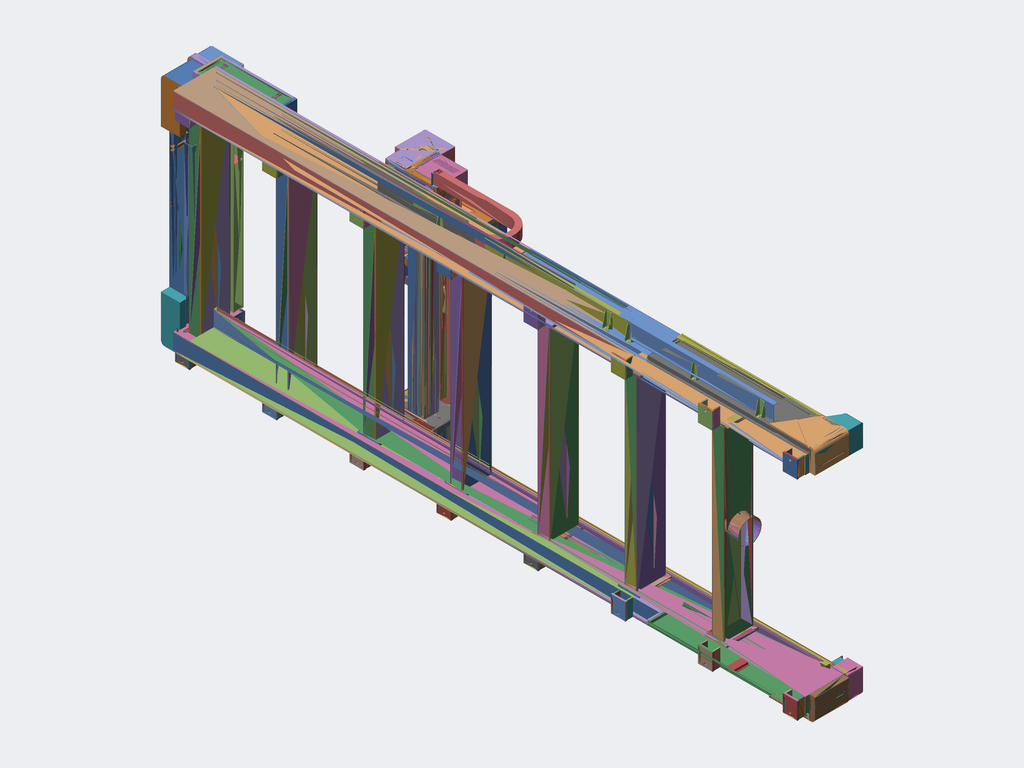Assembly | SolidWorks | 145 different items | 188 placed
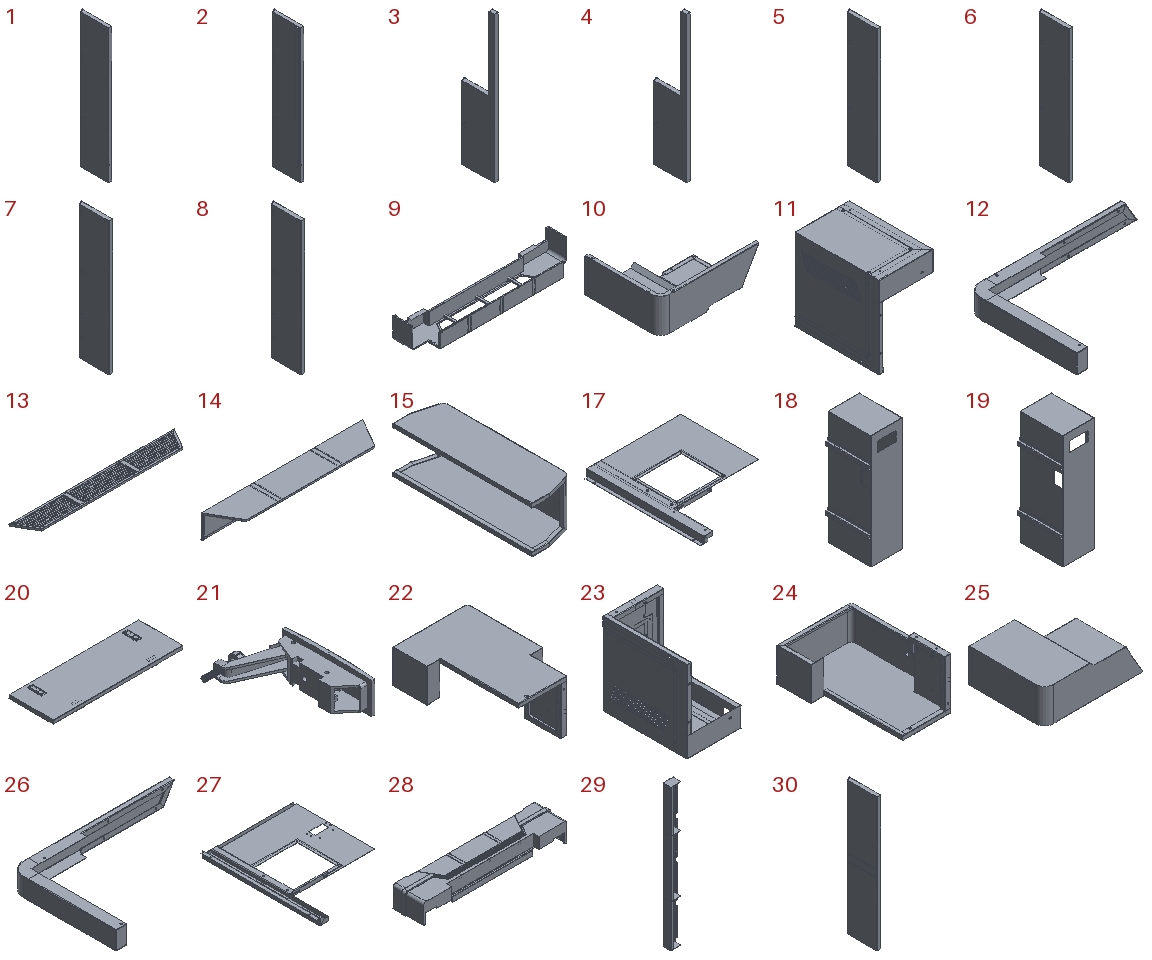Parts list (item | name | quantity | parent item | size | volume | features):
1 | (subassembly) | x1 | in 2 | 50 x 430 x 1914 mm | 1681959 mm3 | -
2 | (subassembly) | x1 | - | 70 x 430 x 1914 mm | 2035587 mm3 | -
3 | (subassembly) | x1 | in 4 | 50 x 430 x 1800 mm | 1098958 mm3 | -
4 | (subassembly) | x1 | - | 50 x 430 x 1800 mm | 1098958 mm3 | -
5 | (subassembly) | x1 | in 6 | 50 x 430 x 1800 mm | 1586446 mm3 | -
6 | (subassembly) | x1 | - | 50 x 430 x 1800 mm | 1586446 mm3 | -
7 | (subassembly) | x1 | in 8 | 50 x 430 x 1800 mm | 1585936 mm3 | -
8 | (subassembly) | x1 | - | 50 x 430 x 1800 mm | 1585936 mm3 | -
9 | (subassembly) | x1 | in 28 | 2780 x 555 x 380 mm | 4361230 mm3 | features ReferencePattern 7, MirrorCompFeat 2, LocalLPattern 1
10 | (subassembly) | x1 | in 28 | 540.3 x 413 x 185.75 mm | 547787 mm3 | -
11 | (subassembly) | x1 | - | 245 x 380 x 370 mm | 729240 mm3 | features InContextFeatHolder 20
12 | (subassembly) | x1 | in 28 | 600.7 x 400 x 70 mm | 210218 mm3 | -
13 | (subassembly) | x1 | in 28 | 1758 x 220 x 20 mm | 727420 mm3 | features LocalLPattern 1, ReferencePattern 1
14 | (subassembly) | x1 | in 28 | 1885 x 336.9 x 273 mm | 1993401 mm3 | features ReferencePattern 2, LocalLPattern 1
15 | (subassembly) | x1 | in 16 | 229.9 x 723 x 240 mm | 1145604 mm3 | features MirrorCompFeat 2, ReferencePattern 2
16 | (subassembly) | x1 | - | - | - | features CompositeCurve 3, MirrorCompFeat 1, ReferencePattern 1
17 | (subassembly) | x1 | in 16 | 600 x 723 x 41.7 mm | 569588 mm3 | -
18 | (subassembly) | x1 | - | 275.9 x 340 x 900 mm | 2191586 mm3 | -
19 | (subassembly) | x1 | in 18 | 270 x 340 x 900 mm | 1657617 mm3 | features MirrorCompFeat 1, ReferencePattern 1
20 | (subassembly) | x1 | in 18 | 834 x 286 x 75.7 mm | 533972 mm3 | features ReferencePattern 2, MirrorCompFeat 1
21 | (subassembly) | x2 | in 20 | 75.7 x 110.704 x 34.425 mm | 27643 mm3 | -
22 | (subassembly) | x1 | - | 355 x 533 x 245 mm | 625684 mm3 | -
23 | (subassembly) | x1 | - | 245 x 380 x 370 mm | 729240 mm3 | -
24 | (subassembly) | x1 | - | 355 x 533 x 245 mm | 625684 mm3 | -
25 | (subassembly) | x1 | in 28 | 540.3 x 413 x 185.75 mm | 547787 mm3 | -
26 | (subassembly) | x1 | in 28 | 600.7 x 400 x 70 mm | 210218 mm3 | -
27 | (subassembly) | x1 | in 16 | 600 x 723 x 41.7 mm | 564160 mm3 | -
28 | (subassembly) | x1 | - | - | 9484925 mm3 | features ReferencePattern 2, MirrorCompFeat 1
29 | (subassembly) | x1 | - | 184 x 120 x 2170 mm | 2640539 mm3 | features LocalLPattern 2, ReferencePattern 2
30 | (subassembly) | x3 | in 31 | 50 x 430 x 1800 mm | 1681113 mm3 | -
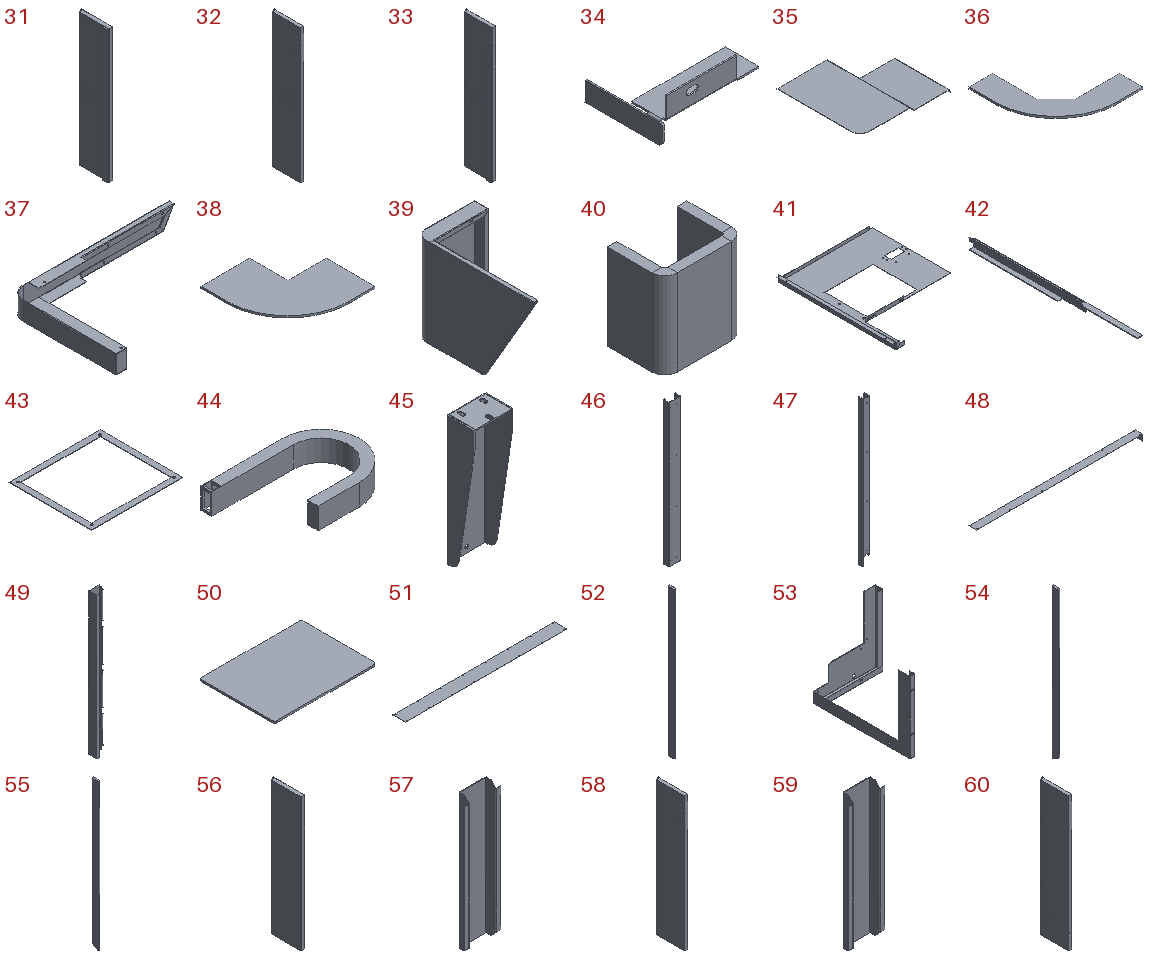31 | (subassembly) | x3 | - | 70 x 430 x 1800 mm | 2368428 mm3 | -
32 | (subassembly) | x1 | in 33 | 50 x 430 x 1914 mm | 1776618 mm3 | -
33 | (subassembly) | x1 | - | 70 x 430 x 1914 mm | 2130249 mm3 | -
34 | - | x1 | in 22 | 86.5 x 70 x 38.5 mm | 7275 mm3 | features ICE 4, Fillet 2, EdgeFlange 1, FlatPattern 1, SMBaseFlange 1, SMMiteredFlange 1, SheetMetal 1
35 | - | x1 | in 25 | 452.1 x 411.5 x 35.646 mm | 260471 mm3 | features MirrorStock 1
36 | - | x1 | in 25 | 68.3 x 68.3 x 1.5 mm | 2665 mm3 | features MirrorStock 1
37 | - | x1 | in 26 | 600.7 x 400 x 70 mm | 200425 mm3 | features MirrorStock 1
38 | - | x2 | in 26 | 68.3 x 68.3 x 1.5 mm | 4896 mm3 | features MirrorStock 1
39 | - | x1 | - | 270 x 544 x 405.75 mm | 580756 mm3 | features MirrorStock 1
40 | - | x1 | in 24 | 25 x 18 x 27 mm | 4281 mm3 | features MirrorStock 1
41 | - | x1 | in 27 | 600 x 723 x 41.7 mm | 400896 mm3 | features Cut 2, ICE 1, MirrorStock 1
42 | - | x1 | in 27 | 22.5 x 718.5 x 47 mm | 130417 mm3 | features 3DProfileFeature 2, MirrorStock 1
43 | - | x1 | in 27 | 310 x 281.5 x 1.5 mm | 32848 mm3 | features MirrorStock 1
44 | - | x1 | - | 732.5 x 465 x 130 mm | 10613161 mm3 | features ICE 3, Extrusion 1
45 | - | x1 | - | 70 x 50 x 232 mm | 69334 mm3 | features ICE 3, EdgeFlange 1, Fillet 1, FlatPattern 1, SMBaseFlange 1, SheetMetal 1
46 | - | x1 | - | 180 x 80 x 2190 mm | 1160945 mm3 | features ICE 2, LPattern 2, SMMiteredFlange 2, Chamfer 1, Fillet 1, FlatPattern 1, SMBaseFlange 1, SheetMetal 1
47 | - | x1 | - | 100 x 80 x 2323 mm | 934752 mm3 | features ICE 5, Fillet 2, LPattern 2, SMBaseFlange 2, Chamfer 1, FlatPattern 1, SheetMetal 1
48 | - | x1 | - | 2196 x 100 x 80 mm | 339571 mm3 | features Fillet 1, FlatPattern 1, ICE 1, LPattern 1, SMBaseFlange 1, SMMiteredFlange 1, SheetMetal 1
49 | - | x1 | in 29 | 184 x 120 x 2170 mm | 2431565 mm3 | features ICE 2, EdgeFlange 1, FlatPattern 1, LPattern 1, SMBaseFlange 1, SheetMetal 1
50 | - | x4 | in 29 | 153.5 x 113.5 x 3 mm | 52244 mm3 | features Extrusion 1, Fillet 1
51 | - | x1 | - | 2232 x 176 x 1.5 mm | 587982 mm3 | features Fillet 1, FlatPattern 1, ICE 1, LPattern 1, SMBaseFlange 1, SheetMetal 1
52 | - | x3 | in 31 | 20 x 70 x 1800 mm | 385797 mm3 | features EdgeFlange 2, FlatPattern 1, ICE 1, LPattern 1, SMBaseFlange 1, SheetMetal 1
53 | - | x1 | in 11 | 245 x 380 x 280 mm | 150537 mm3 | features ICE 15, SMMiteredFlange 7, LPattern 2, Cut 1, EdgeFlange 1, Fillet 1, FlatPattern 1, SMBaseFlange 1, SheetMetal 1
54 | - | x1 | in 33 | 20 x 70 x 1667 mm | 353631 mm3 | features ICE 8, EdgeFlange 2, FlatPattern 1, LPattern 1, SMBaseFlange 1, SheetMetal 1
55 | - | x1 | in 2 | 20 x 70 x 1667 mm | 353629 mm3 | features ICE 7, EdgeFlange 3, FlatPattern 1, LPattern 1, SMBaseFlange 1, SheetMetal 1
56 | - | x3 | in 30 | 50 x 430 x 1800 mm | 1586957 mm3 | features EdgeFlange 5, ICE 4, LPattern 3, Fillet 1, FlatPattern 1, SMBaseFlange 1, SMMiteredFlange 1, SheetMetal 1
57 | - | x3 | in 30 | 107 x 30.5 x 395 mm | 94156 mm3 | features FlatPattern 1, ICE 1, SMBaseFlange 1, SheetMetal 1
58 | - | x1 | in 32 | 50 x 430 x 1914 mm | 1682462 mm3 | features ICE 7, EdgeFlange 5, LPattern 3, Cut 1, Fillet 1, FlatPattern 1, SMBaseFlange 1, SMMiteredFlange 1, SheetMetal 1
59 | - | x1 | in 32 | 107 x 30.5 x 395 mm | 94156 mm3 | features FlatPattern 1, ICE 1, SMBaseFlange 1, SheetMetal 1
60 | - | x1 | in 1 | 50 x 430 x 1914 mm | 1681959 mm3 | features ICE 7, EdgeFlange 5, LPattern 4, Cut 3, Fillet 1, FlatPattern 1, SMBaseFlange 1, SMMiteredFlange 1, SheetMetal 1
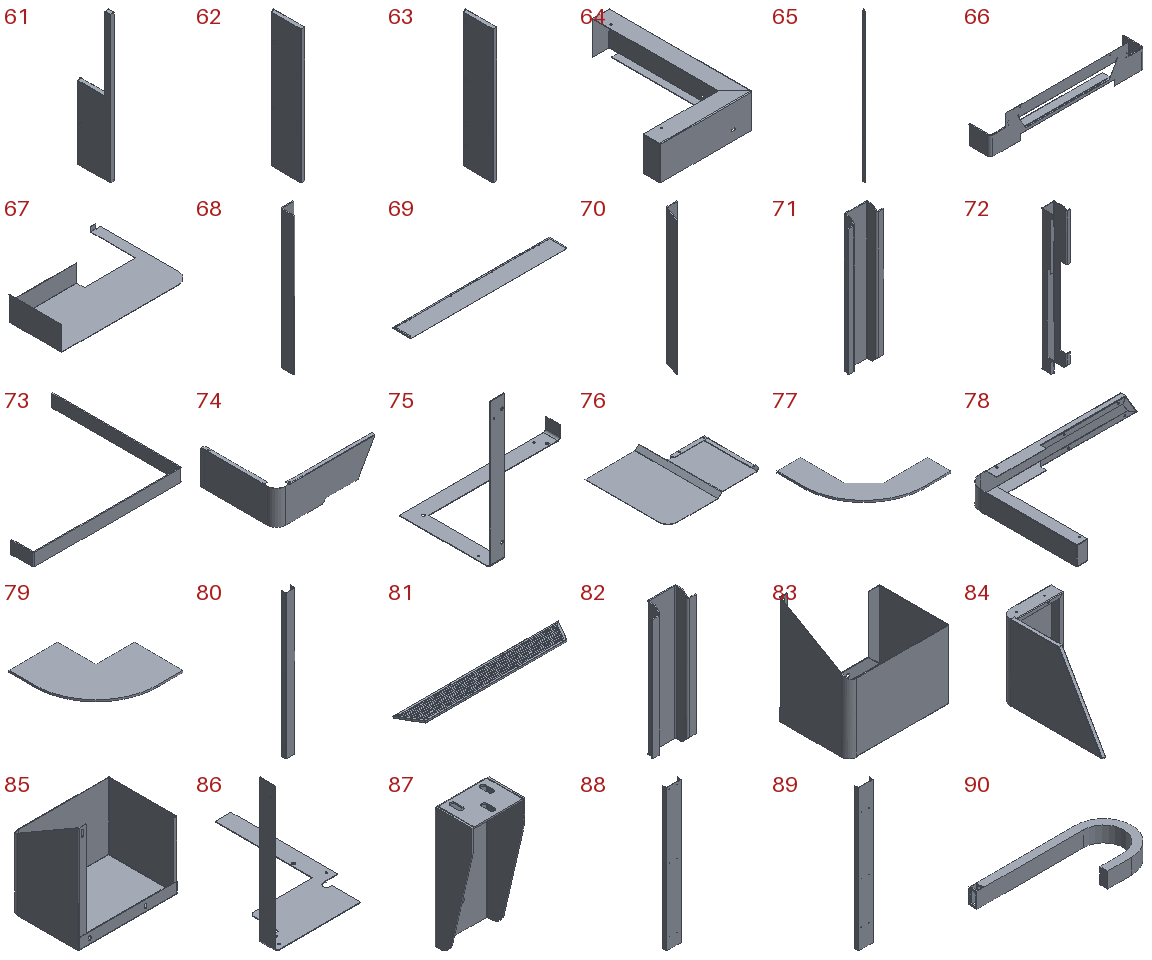61 | - | x1 | in 3 | 50 x 430 x 1800 mm | 1098958 mm3 | features EdgeFlange 7, ICE 5, LPattern 4, Cut 2, Fillet 2, FlatPattern 1, SMBaseFlange 1, SMMiteredFlange 1, SheetMetal 1
62 | - | x1 | in 5 | 50 x 430 x 1800 mm | 1586446 mm3 | features EdgeFlange 5, ICE 4, LPattern 4, Cut 1, Fillet 1, FlatPattern 1, SMBaseFlange 1, SMMiteredFlange 1, SheetMetal 1
63 | - | x1 | in 7 | 50 x 430 x 1800 mm | 1585936 mm3 | features EdgeFlange 5, ICE 4, LPattern 4, Cut 3, Fillet 1, FlatPattern 1, SMBaseFlange 1, SMMiteredFlange 1, SheetMetal 1
64 | - | x1 | in 11 | 245 x 380 x 90 mm | 139211 mm3 | features ICE 5, EdgeFlange 1, FlatPattern 1, SMBaseFlange 1, SMMiteredFlange 1, SheetMetal 1
65 | - | x3 | in 31 | 24 x 42 x 1700 mm | 301518 mm3 | features ICE 2, Fillet 1, FlatPattern 1, LPattern 1, SMBaseFlange 1, SheetMetal 1
66 | - | x1 | in 9 | 2780 x 380 x 555 mm | 2537255 mm3 | features ICE 20, EdgeFlange 8, SMBaseFlange 5, LPattern 3, MirrorPattern 2, FlatPattern 1, SheetMetal 1
67 | - | x1 | in 9 | 540.3 x 378.5 x 101.5 mm | 241079 mm3 | features EdgeFlange 2, FlatPattern 1, SMBaseFlange 1, SMMiteredFlange 1, SheetMetal 1
68 | - | x2 | in 9 | 18.5 x 20 x 201.5 mm | 11021 mm3 | features FlatPattern 1, SMBaseFlange 1, SheetMetal 1
69 | - | x1 | in 9 | 2210 x 251.5 x 20 mm | 975971 mm3 | features ICE 6, EdgeFlange 2, MirrorPattern 2, FlatPattern 1, LPattern 1, SMBaseFlange 1, SheetMetal 1
70 | - | x1 | in 9 | 20 x 20 x 269.592 mm | 14701 mm3 | features ICE 3, SMBaseFlange 2, EdgeFlange 1, FlatPattern 1, SheetMetal 1
71 | - | x3 | in 9 | 61 x 18.5 x 232.5 mm | 31420 mm3 | features FlatPattern 1, ICE 1, SMBaseFlange 1, SheetMetal 1
72 | - | x3 | in 9 | 61 x 40 x 433 mm | 65237 mm3 | features ICE 2, FlatPattern 1, SMBaseFlange 1, SheetMetal 1
73 | - | x1 | in 9 | 220 x 191 x 18.5 mm | 12216 mm3 | features FlatPattern 1, SMBaseFlange 1, SheetMetal 1
74 | - | x1 | in 10 | 540.3 x 413 x 185.75 mm | 284651 mm3 | features ICE 10, EdgeFlange 4, Chamfer 1, FlatPattern 1, Hem 1, SMBaseFlange 1, SheetMetal 1
75 | - | x1 | in 11 | 353.5 x 218.5 x 348.5 mm | 47454 mm3 | features Cut 5, EdgeFlange 2, FlatPattern 1, SMBaseFlange 1, SheetMetal 1
76 | - | x1 | in 10 | 452.1 x 411.5 x 35.646 mm | 260471 mm3 | features ICE 4, EdgeFlange 2, SMBaseFlange 2, SMMiteredFlange 2, Fillet 1, FlatPattern 1, Jog 1, SheetMetal 1
77 | - | x1 | in 10 | 68.3 x 68.3 x 1.5 mm | 2665 mm3 | features Extrusion 1
78 | - | x1 | in 12 | 600.7 x 400 x 70 mm | 200425 mm3 | features ICE 10, EdgeFlange 4, SMMiteredFlange 2, FlatPattern 1, SMBaseFlange 1, SheetMetal 1
79 | - | x2 | in 12 | 68.3 x 68.3 x 1.5 mm | 4896 mm3 | features FlatPattern 1, SMBaseFlange 1, SheetMetal 1
80 | - | x1 | in 28 | 100 x 50 x 1550 mm | 886864 mm3 | features ICE 2, LPattern 2, FlatPattern 1, SMBaseFlange 1, SheetMetal 1
81 | - | x1 | in 13 | 1758 x 220 x 20 mm | 678104 mm3 | features ICE 19, LPattern 12, EdgeFlange 4, FlatPattern 1, SMBaseFlange 1, SheetMetal 1
82 | - | x2 | in 13 | 61 x 18.5 x 183.5 mm | 24658 mm3 | features FlatPattern 1, ICE 1, SMBaseFlange 1, SheetMetal 1
83 | - | x1 | - | 265 x 184 x 285 mm | 277384 mm3 | features ICE 5, EdgeFlange 2, SMBaseFlange 2, FlatPattern 1, SMMiteredFlange 1, SheetMetal 1
84 | - | x1 | - | 270 x 544 x 405.75 mm | 580756 mm3 | features ICE 17, EdgeFlange 7, SMBaseFlange 6, LPattern 2, FlatPattern 1, SheetMetal 1
85 | - | x1 | - | 265 x 184 x 285 mm | 272700 mm3 | features ICE 5, EdgeFlange 2, SMBaseFlange 2, SMMiteredFlange 2, FlatPattern 1, LPattern 1, SheetMetal 1
86 | - | x1 | in 11 | 218.5 x 316.5 x 318.5 mm | 52403 mm3 | features Cut 6, EdgeFlange 1, Fillet 1, FlatPattern 1, SMBaseFlange 1, SheetMetal 1
87 | - | x9 | - | 70 x 50 x 160 mm | 49876 mm3 | features ICE 3, EdgeFlange 1, Fillet 1, FlatPattern 1, SMBaseFlange 1, SheetMetal 1
88 | - | x1 | - | 180 x 45 x 1715 mm | 683780 mm3 | features LPattern 2, Chamfer 1, FlatPattern 1, ICE 1, SMBaseFlange 1, SheetMetal 1
89 | - | x1 | - | 180 x 45 x 1715 mm | 683780 mm3 | features Chamfer 2, ICE 2, LPattern 2, FlatPattern 1, SMBaseFlange 1, SheetMetal 1
90 | - | x1 | - | 1128 x 465 x 130 mm | 13528411 mm3 | features ICE 3, Extrusion 1
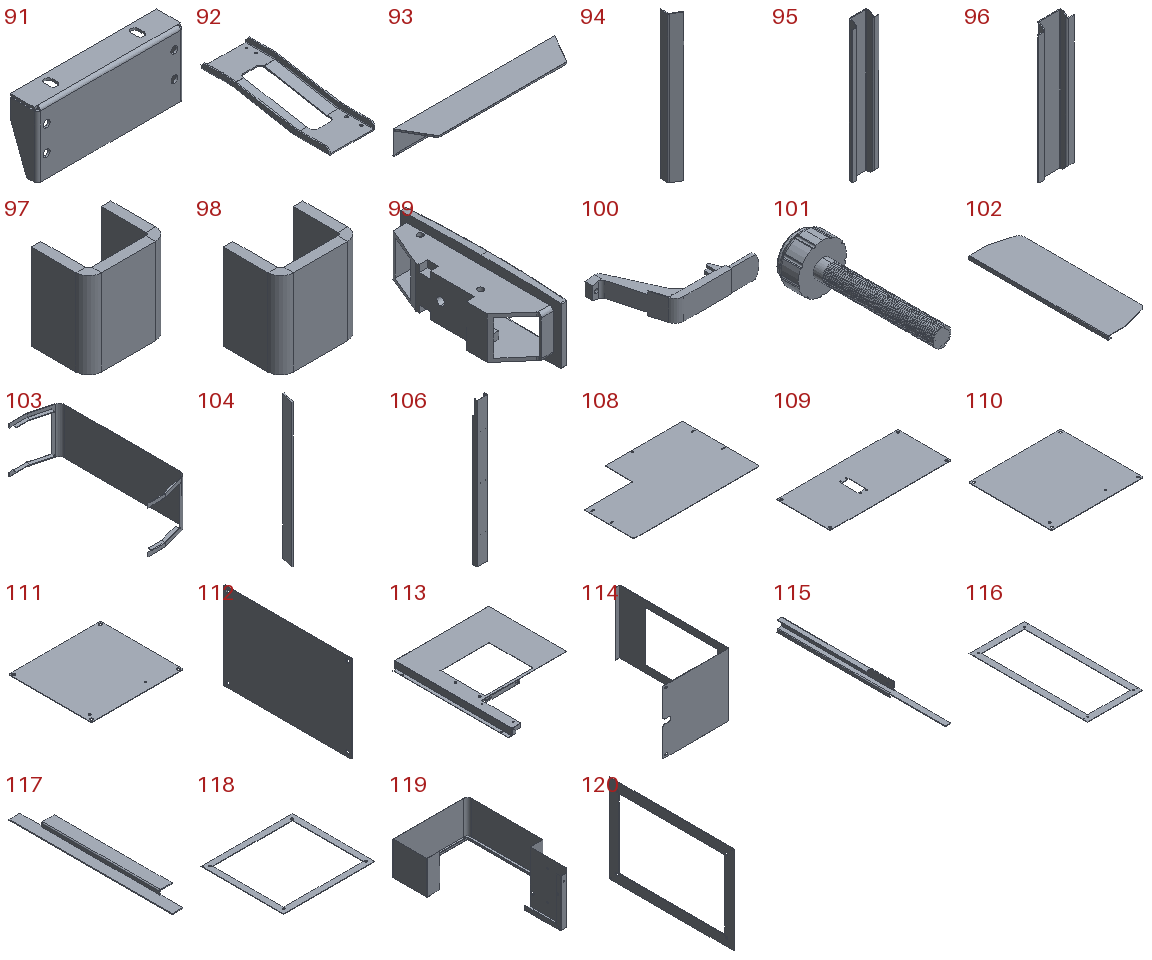91 | - | x2 | in 16 | 135 x 25 x 60 mm | 25438 mm3 | features ICE 5, SMBaseFlange 2, EdgeFlange 1, FlatPattern 1, LPattern 1, SheetMetal 1
92 | - | x1 | in 16 | 124 x 345 x 47 mm | 120902 mm3 | features Chamfer 1, EdgeFlange 1, FlatPattern 1, Jog 1, SMBaseFlange 1, SheetMetal 1
93 | - | x1 | in 14 | 1885 x 336.9 x 273 mm | 1826006 mm3 | features ICE 8, EdgeFlange 6, SMBaseFlange 5, SMMiteredFlange 2, FlatPattern 1, SheetMetal 1
94 | - | x2 | in 14 | 17.897 x 24.1 x 251.3 mm | 12439 mm3 | features FlatPattern 1, SMBaseFlange 1, SheetMetal 1
95 | - | x2 | in 14 | 61 x 18.5 x 317 mm | 43080 mm3 | features FlatPattern 1, ICE 1, SMBaseFlange 1, SheetMetal 1
96 | - | x2 | in 14 | 61 x 13.5 x 234.5 mm | 28178 mm3 | features FlatPattern 1, ICE 1, SMBaseFlange 1, SheetMetal 1
97 | - | x1 | in 11 | 25 x 18 x 27 mm | 4281 mm3 | features FlatPattern 1, SMBaseFlange 1, SheetMetal 1
98 | - | x1 | in 22 | 25 x 18 x 27 mm | 4281 mm3 | features FlatPattern 1, SMBaseFlange 1, SheetMetal 1
99 | - | x2 | in 21 | 26.6 x 92.8 x 34.425 mm | 14657 mm3 | features BaseBody 1
100 | - | x2 | in 21 | 100.61 x 62 x 20.1 mm | 11692 mm3 | features BaseBody 1
101 | - | x2 | in 21 | 12.8 x 38.7 x 12.78 mm | 1300 mm3 | features BaseBody 1
102 | - | x2 | in 15 | 227.9 x 719 x 20 mm | 367716 mm3 | features EdgeFlange 2, FlatPattern 1, SMBaseFlange 1, SheetMetal 1
103 | - | x1 | in 15 | 229.9 x 723 x 240 mm | 395484 mm3 | features EdgeFlange 2, MirrorPattern 2, FlatPattern 1, ICE 1, SMBaseFlange 1, SheetMetal 1
104 | - | x2 | in 15 | 6.591 x 17.904 x 204 mm | 7344 mm3 | features Extrusion 1
105 | - | x1 | - | - | - | features BaseBody 540, RefSurface 319
106 | - | x1 | - | 180 x 80 x 2507 mm | 1382139 mm3 | features EdgeFlange 6, ICE 3, Cut 2, Chamfer 1, FlatPattern 1, LPattern 1, SMBaseFlange 1, SheetMetal 1
107 | - | x1 | in 16 | - | - | features BaseBody 411, RefSurface 73, ICE 2
108 | - | x1 | - | 608.5 x 375 x 1.5 mm | 294054 mm3 | features ICE 3, LPattern 2, FlatPattern 1, SMBaseFlange 1, SheetMetal 1
109 | - | x1 | in 16 | 538.2 x 238 x 1.5 mm | 187659 mm3 | features HoleWzd 2, Cut 1, Extrusion 1, Fillet 1, ICE 1
110 | - | x1 | in 16 | 296 x 267.5 x 1.5 mm | 118387 mm3 | features Chamfer 1, Cut 1, Extrusion 1, Fillet 1, ICE 1
111 | - | x1 | in 16 | 296 x 267.5 x 1.5 mm | 118337 mm3 | features Cut 1, Extrusion 1, Fillet 1, HoleWzd 1
112 | - | x1 | in 16 | 1.5 x 316.6 x 216.5 mm | 102468 mm3 | features HoleWzd 2, Extrusion 1, Fillet 1
113 | - | x1 | in 17 | 600 x 723 x 41.7 mm | 406324 mm3 | features ICE 8, EdgeFlange 5, LPattern 4, Cut 1, FlatPattern 1, SMBaseFlange 1, SheetMetal 1
114 | - | x1 | in 16 | 291.5 x 482 x 276.8 mm | 222164 mm3 | features ICE 2, Cut 1, EdgeFlange 1, Fillet 1, FlatPattern 1, LPattern 1, SMBaseFlange 1, SheetMetal 1
115 | - | x1 | in 17 | 22.5 x 718.5 x 47 mm | 130417 mm3 | features EdgeFlange 3, 3DProfileFeature 2, Cut 1, FlatPattern 1, ICE 1, SMBaseFlange 1, SheetMetal 1
116 | - | x1 | in 16 | 260 x 560.2 x 1.5 mm | 68162 mm3 | features Cut 2, FlatPattern 1, LPattern 1, SMBaseFlange 1, SheetMetal 1
117 | - | x1 | in 16 | 38.3 x 276.6 x 8.5 mm | 15431 mm3 | features EdgeFlange 2, FlatPattern 1, SMBaseFlange 1, SheetMetal 1
118 | - | x1 | in 17 | 310 x 281.5 x 1.5 mm | 32848 mm3 | features Cut 1, FlatPattern 1, ICE 1, SMBaseFlange 1, SheetMetal 1
119 | - | x1 | in 22 | 355 x 533 x 245 mm | 356884 mm3 | features ICE 14, EdgeFlange 4, SMMiteredFlange 3, SMBaseFlange 2, Cut 1, Fillet 1, FlatPattern 1, LPattern 1, SheetMetal 1
120 | - | x1 | in 16 | 1.5 x 338.6 x 238.5 mm | 39286 mm3 | features Extrusion 1
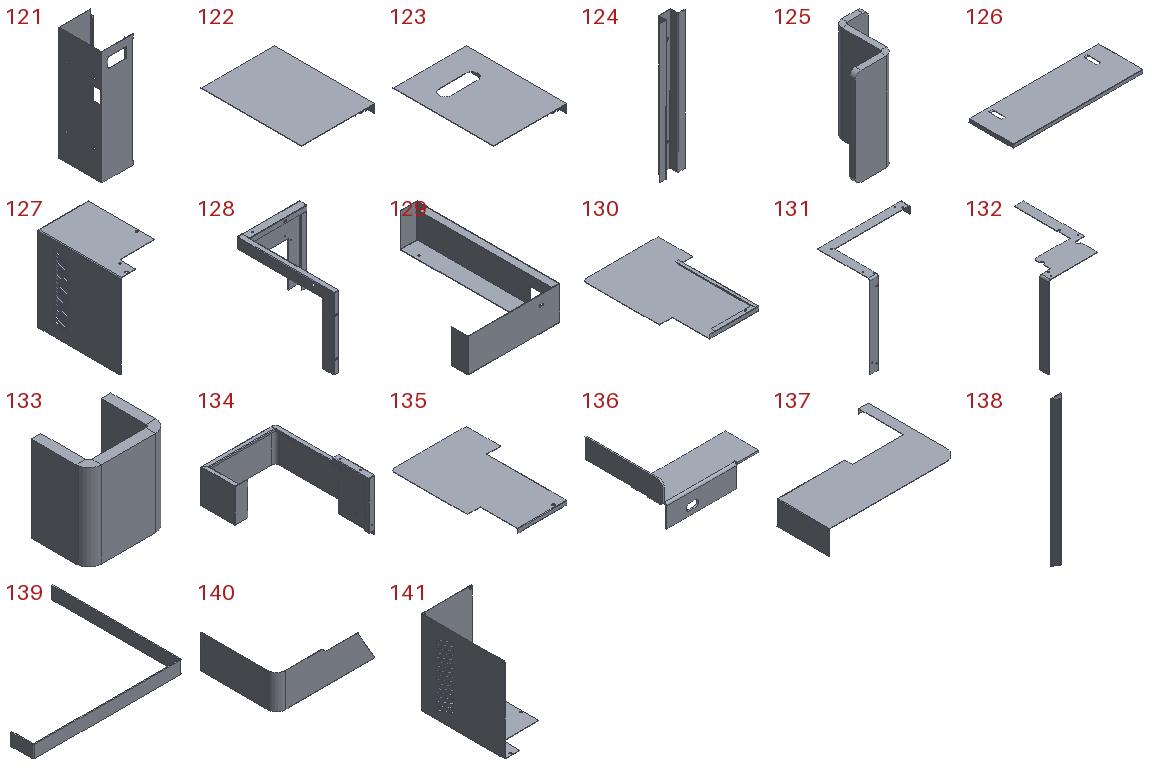121 | - | x1 | in 19 | 250 x 340 x 900 mm | 1255343 mm3 | features EdgeFlange 6, Cut 3, FlatPattern 1, LPattern 1, SMBaseFlange 1, SheetMetal 1
122 | - | x1 | in 19 | 248.5 x 337 x 47 mm | 155691 mm3 | features EdgeFlange 3, FlatPattern 1, SMBaseFlange 1, SheetMetal 1
123 | - | x1 | in 19 | 248.5 x 337 x 47 mm | 148406 mm3 | features EdgeFlange 3, Cut 1, FlatPattern 1, SMBaseFlange 1, SheetMetal 1
124 | - | x2 | in 19 | 63 x 20 x 340 mm | 49088 mm3 | features Cut 1, FlatPattern 1, LPattern 1, SMBaseFlange 1, SheetMetal 1
125 | - | x2 | in 20 | 32 x 28 x 50 mm | 8205 mm3 | features Fillet 1, FlatPattern 1, SMBaseFlange 1, SheetMetal 1
126 | - | x1 | in 20 | 834 x 286 x 23 mm | 462099 mm3 | features EdgeFlange 2, FlatPattern 1, ICE 1, MirrorPattern 1, SMBaseFlange 1, SheetMetal 1
127 | - | x1 | in 23 | 199 x 329 x 334 mm | 335353 mm3 | features MirrorStock 1
128 | - | x1 | in 23 | 245 x 380 x 280 mm | 150537 mm3 | features MirrorStock 1
129 | - | x1 | in 23 | 245 x 380 x 90 mm | 139211 mm3 | features MirrorStock 1
130 | - | x1 | in 22 | 352 x 531.5 x 20 mm | 257244 mm3 | features ICE 4, EdgeFlange 3, Fillet 1, FlatPattern 1, SMBaseFlange 1, SMMiteredFlange 1, SheetMetal 1
131 | - | x1 | in 23 | 353.5 x 218.5 x 348.5 mm | 47454 mm3 | features MirrorStock 1
132 | - | x1 | in 23 | 218.5 x 316.5 x 318.5 mm | 52403 mm3 | features MirrorStock 1
133 | - | x1 | in 23 | 25 x 18 x 27 mm | 4281 mm3 | features MirrorStock 1
134 | - | x1 | in 24 | 355 x 533 x 245 mm | 356884 mm3 | features MirrorStock 1
135 | - | x1 | in 24 | 352 x 531.5 x 20 mm | 257244 mm3 | features MirrorStock 1
136 | - | x1 | in 24 | 86.5 x 70 x 38.5 mm | 7275 mm3 | features MirrorStock 1
137 | - | x1 | in 9 | 540.3 x 378.5 x 101.5 mm | 241079 mm3 | features MirrorStock 1
138 | - | x1 | in 9 | 20 x 20 x 269.592 mm | 14701 mm3 | features MirrorStock 1
139 | - | x1 | in 9 | 220 x 191 x 18.5 mm | 12216 mm3 | features MirrorStock 1
140 | - | x1 | in 25 | 540.3 x 413 x 185.75 mm | 284651 mm3 | features MirrorStock 1
141 | - | x1 | in 11 | 199 x 329 x 334 mm | 335353 mm3 | features ICE 6, Chamfer 2, Fillet 2, EdgeFlange 1, FlatPattern 1, LPattern 1, SMBaseFlange 1, SheetMetal 1
142 | RW Side Front Trim Plate | x1 | - | - | - | -
143 | RW Side Plate 1 Rib Plate | x1 | - | - | - | -
144 | RW Side Plate 3 Rib Plate | x1 | - | - | - | -
145 | RW Side Plate Hanger 1 | x1 | - | - | - | -
Mates (type | each side: item.copy, entity, surface, feature):
In the top assembly
Coincident | assembly face | assembly face | 10 times
DistanceDim | assembly face | assembly face
Width | assembly face | assembly face | assembly face | assembly face
Coincident | assembly face | 49.1 face plane Base-Flange 1 | 2 times
Width | 50.1 face plane Boss-Extrude 1 | 50.2 face plane Boss-Extrude 1 | assembly face | assembly face
Coincident | 93.1 face plane Edge-Flange 1 | 49.1 face plane Base-Flange 1
Width | 66.1 face plane Base-Flange 1 | 66.1 face plane Base-Flange 1 | assembly face | assembly face
Coincident | assembly face | 80.1 face plane Base-Flange 1
Coincident | 137.1 face plane RW Front Lower Corner Wrap Weld 2(Modified) Mirror | 56.1 face plane Base-Flange 1
DistanceDim | 56.1 edge | assembly face
Coincident | 56.1 face plane Edge-Flange 5 | assembly face
Width | assembly face | assembly face | 57.1 face plane Base-Flange 1 | 57.1 face plane Base-Flange 1
DistanceDim | 56.1 face plane Edge-Flange 3 | 66.1 face plane Edge-Flange 14
Coincident | assembly face | 84.1 face plane Edge-Flange 8
Coincident | 54.1 face plane Base-Flange 1 | 84.1 face plane Edge-Flange 6
Coincident | 58.1 face plane Base-Flange 1 | 84.1 face plane Edge-Flange 4
Coincident | assembly face | 58.1 face plane Edge-Flange 1
Coincident | 56.1 face plane Base-Flange 1 | assembly face
DistanceDim | assembly face | 56.1 face plane Edge-Flange 1
Slot | 85.1 face cylinder Cut-Extrude 3 | 58.1 face cylinder Cut-Extrude 10 | 2 times
Coincident | 58.1 face plane Base-Flange 1 | 56.2 face plane Base-Flange 1
Coincident | 84.1 face plane Edge-Flange 6 | 85.1 face plane Edge-Flange 2
Parallel | 84.1 face plane Base-Flange 1 | 85.1 face plane Edge-Flange 1
Coincident | 67.1 face plane Base-Flange 1 | assembly face
DistanceDim | assembly face | 66.1 face plane Edge-Flange 14
Coincident | assembly face | 83.1 face plane Edge-Flange 4
DistanceDim | 83.1 face plane Edge-Flange 2 | assembly face
DistanceDim | 83.1 face plane Base-Flange 1 | assembly face
Coincident | 60.1 face plane Base-Flange 1 | 87.1 face plane Edge-Flange 1
DistanceDim | 87.1 face plane Base-Flange 1 | 60.1 face plane Base-Flange 1
Coincident | 88.1 face plane Base-Flange 1 | 90.1 face plane Boss-Extrude 1
Width | 90.1 face plane Boss-Extrude 1 | 90.1 face plane Boss-Extrude 1 | 89.1 face plane Base-Flange 1 | 89.1 face plane Base-Flange 1
DistanceDim | 90.1 face plane Boss-Extrude 1 | assembly face
Coincident | 88.1 face plane Base-Flange 1 | assembly face | 2 times
Coincident | 88.1 face plane Base-Flange 1 | 106.1 face plane Base-Flange 1 | 2 times
DistanceDim | 88.1 face plane Base-Flange 1 | 87.1 face plane Base-Flange 1
DistanceDim | 88.1 face plane Base-Flange 1 | 89.1 face plane Base-Flange 1
Coincident | 88.1 face plane Base-Flange 1 | 89.1 face plane Base-Flange 1 | 2 times
DistanceDim | 61.1 face plane Base-Flange 1 | assembly face
DistanceDim | 62.1 face plane Base-Flange 1 | assembly face
DistanceDim | 62.1 face plane Edge-Flange 1 | 61.1 face plane Edge-Flange 3
DistanceDim | 63.1 face plane Edge-Flange 1 | 62.1 face plane Edge-Flange 3
Coincident | 62.1 face plane Base-Flange 1 | 63.1 face plane Base-Flange 1
Coincident | 63.1 face plane Base-Flange 1 | 87.2 face plane Edge-Flange 1
Coincident | 87.3 face plane Edge-Flange 1 | 87.2 face plane Edge-Flange 1
DistanceDim | 87.2 face plane Base-Flange 1 | 87.3 face plane Base-Flange 1
Coincident | 106.1 face plane Edge-Flange 3 | 51.1 face plane Base-Flange 1
Coincident | 106.1 edge | 51.1 face plane Base-Flange 1
DistanceDim | 51.1 face plane Base-Flange 1 | 106.1 face plane Base-Flange 1
DistanceDim | 122.1 face plane Base-Flange 1 | 66.1 face plane Edge-Flange 14
Coincident | assembly face | 124.1 face plane Base-Flange 1
DistanceDim | 121.1 face plane Base-Flange 1 | 61.1 face plane Edge-Flange 6
Coincident | 63.1 face plane Base-Flange 1 | 87.4 face plane Edge-Flange 1
Coincident | 89.1 face plane Base-Flange 1 | 87.4 face plane Base-Flange 1
DistanceDim | 87.4 face plane Base-Flange 1 | 89.1 face plane Base-Flange 1
Coincident | assembly face | 45.1 face plane Edge-Flange 1
DistanceDim | 45.1 face plane Base-Flange 1 | assembly face | 2 times
Coincident | 46.1 face plane Base-Flange 1 | 45.1 face plane Base-Flange 1
Concentric | 46.1 edge | 45.1 face cylinder Cut-Extrude 2 | 2 times
Coincident | 46.1 face plane Base-Flange 1 | 44.1 face plane Boss-Extrude 1
Width | 44.1 face plane Boss-Extrude 1 | 44.1 face plane Boss-Extrude 1 | 46.1 face plane Base-Flange 1 | 46.1 face plane Base-Flange 1
Coincident | assembly face | 107.1 face | 2 times
Coincident | 44.1 face plane Boss-Extrude 1 | 41.1 face plane Head Cover Weldment 1 Mirror
DistanceDim | 119.1 face plane Edge-Flange 13 | assembly face
Coincident | assembly face | 130.1 face plane Miter Flange 1
Coincident | assembly face | 53.1 face plane Miter Flange 4
Coincident | assembly face | 53.1 face plane Miter Flange 5
Coincident | assembly face | 119.1 face plane Edge-Flange 2
Coincident | assembly face | 53.1 face plane Edge-Flange 1
Coincident | 53.1 face plane Miter Flange 11 | 108.1 face plane Base-Flange 1
Coincident | 34.1 face plane Base-Flange 1 | 108.1 face plane Base-Flange 1
Coincident | 119.1 face plane Base-Flange 1 | 108.1 face plane Base-Flange 1
Coincident | 128.1 face plane RW13015 Left Motor Cover Part 1(New) Mirror | 91.1 face plane Edge-Flange 1
Coincident | 90.1 face plane Boss-Extrude 1 | 91.1 face plane Base-Flange 1
Width | 91.1 face plane Base-Flange 1 | 91.1 face plane Base-Flange 1 | 90.1 face plane Boss-Extrude 1 | 90.1 face plane Boss-Extrude 1
Coincident | 45.1 face plane Base-Flange 1 | 47.1 face plane Base-Flange 1
Slot | 47.1 face plane Cut-Extrude 3 | 45.1 face cylinder Cut-Extrude 2
Parallel | assembly face | 47.1 face plane Base-Flange 1
Coincident | 47.1 face plane Base-Flange 1 | 48.1 face plane Base-Flange 1
Slot | 48.1 face cylinder LPattern 1 | 47.1 face cylinder LPattern 1
Slot | 48.1 face cylinder Cut-Extrude 1 | 47.1 face cylinder Cut-Extrude 1
Coincident | 80.1 face plane Base-Flange 1 | 105.1 face plane Import 96
Coincident | 65.1 face plane Base-Flange 1 | 105.1 face plane Import 38
DistanceDim | 105.1 face plane Import 6 | 61.1 face plane Base-Flange 1
In subassembly 33
Coincident | 58.2 face plane Base-Flange 1 | 54.2 face plane Base-Flange 1 | 2 times
Coincident | 58.2 face plane Edge-Flange 3 | 54.2 face plane Edge-Flange 3
Coincident | 58.2 face plane Base-Flange 1 | 33.1 face | 2 times
DistanceDim | 33.1 face | 58.2 face
Coincident | 58.2 face plane Edge-Flange 5 | 33.1 face
Coincident | 58.2 face plane Miter Flange 1 | 33.1 face
Width | 33.1 face | 33.1 face | 58.2 face plane Edge-Flange 1 | 58.2 face plane Edge-Flange 3
In subassembly 32
Coincident | 58.3 face plane Base-Flange 1 | 59.1 face plane Base-Flange 1 | 2 times
DistanceDim | 59.1 face plane Base-Flange 1 | 58.3 face plane Cut-Extrude 5
Coincident | 58.3 face plane Edge-Flange 5 | 32.1 face
Coincident | 58.3 edge | 32.1 face
In subassembly 29
Coincident | 49.2 face plane Base-Flange 1 | 29.1 face | 6 times
Coincident | 49.2 face plane Base-Flange 1 | 50.3 face plane Boss-Extrude 1 | 3 times
Coincident | 49.2 face plane Base-Flange 1 | 50.4 face plane Boss-Extrude 1 | 3 times
In subassembly 11
Coincident | 64.1 face plane Base-Flange 1 | 53.2 face plane Miter Flange 11
Coincident | 53.2 face plane Miter Flange 9 | 64.1 face plane Base-Flange 1 | 2 times
Coincident | 53.2 face plane Miter Flange 4 | 97.1 face plane Base-Flange 1
Coincident | 53.2 face plane Base-Flange 1 | 97.1 face plane Base-Flange 1
DistanceDim | 53.2 face plane Miter Flange 11 | 97.1 face plane Base-Flange 1
Coincident | 53.2 face plane Cut-Extrude 27 | 64.1 face plane Edge-Flange 1
Coincident | 53.2 face plane Base-Flange 1 | 86.1 face plane Base-Flange 1
DistanceDim | 53.2 face plane Cut-Extrude 22 | 86.1 face plane Base-Flange 1
Coincident | 64.1 face plane Edge-Flange 1 | 75.1 face plane Base-Flange 1
DistanceDim | 75.1 face plane Base-Flange 1 | 64.1 face plane Edge-Flange 1
DistanceDim | 64.1 face plane Edge-Flange 1 | 75.1 face plane Base-Flange 1
Coincident | 75.1 face plane Base-Flange 1 | 141.1 face plane Edge-Flange 1
Coincident | 86.1 face plane Base-Flange 1 | 141.1 face plane Base-Flange 1
Coincident | 86.1 face plane Edge-Flange 1 | 141.1 face plane Edge-Flange 1
DistanceDim | 141.1 face plane Base-Flange 1 | 53.2 face plane Cut-Extrude 22
In subassembly 28
Coincident | 66.2 edge | 28.1 plane
Coincident | 66.2 face plane Base-Flange 1 | 28.1 plane
Coincident | 66.2 face plane Edge-Flange 9 | 81.1 face plane Edge-Flange 12
DistanceDim | 81.1 face plane Edge-Flange 1 | 66.2 face plane Edge-Flange 8
Coincident | 66.2 face plane Base-Flange 1 | 93.2 face plane Miter Flange 2
Coincident | 69.1 face plane Base-Flange 1 | 93.2 face plane Miter Flange 1
Coincident | 93.2 edge | 28.1 plane
Coincident | 69.1 face plane Base-Flange 1 | 76.1 face plane Miter Flange 2
Coincident | 66.2 face plane Base-Flange 1 | 74.1 face plane Edge-Flange 4
Coincident | 66.2 face plane Base-Flange 1 | 74.1 face plane Base-Flange 1
Coincident | 66.2 face plane Base-Flange 1 | 78.1 face plane Edge-Flange 5
Coincident | 74.1 face plane Edge-Flange 3 | 78.1 face plane Edge-Flange 2
DistanceDim | 74.1 face plane Cut-Extrude 7 | 78.1 face cylinder Cut-Extrude 15
Coincident | 13.1 plane | 28.1 plane
Coincident | 66.2 face plane Edge-Flange 6 | 80.2 face plane Base-Flange 1
Parallel | 66.2 face plane Edge-Flange 5 | 80.2 face plane Base-Flange 1
Slot | 80.2 face cylinder LPattern 1 | 66.2 face cylinder Cut-Extrude 19
In subassembly 14
Coincident | 93.3 face plane Miter Flange 1 | 94.1 face plane Base-Flange 1
Coincident | 94.1 face plane Base-Flange 1 | 93.3 face plane Edge-Flange 2
Coincident | 93.3 face plane Edge-Flange 5 | 94.1 face plane Base-Flange 1
Coincident | 93.3 face plane Edge-Flange 5 | 94.2 face plane Base-Flange 1
Coincident | 93.3 face plane Miter Flange 1 | 94.2 face plane Base-Flange 1
Coincident | 93.3 face plane Edge-Flange 2 | 94.2 face plane Base-Flange 1
Coincident | 93.3 face plane Base-Flange 1 | 95.1 face plane Base-Flange 1
Coincident | 93.3 face plane Cut-Extrude 7 | 95.1 face plane Base-Flange 1
Coincident | 93.3 face plane Edge-Flange 1 | 96.1 face plane Base-Flange 1
DistanceDim | 96.1 face plane Base-Flange 1 | 93.3 face plane Cut-Extrude 8
Coincident | 95.1 face plane Base-Flange 1 | 96.1 edge
Width | 95.1 face plane Base-Flange 1 | 95.1 face plane Base-Flange 1 | 93.3 face plane Cut-Extrude 7 | 93.3 face plane Cut-Extrude 7
In subassembly 9
Coincident | 9.1 plane | 66.3 face plane Base-Flange 1
Coincident | 66.3 face plane Base-Flange 1 | 67.2 face plane Base-Flange 1 | 2 times
Coincident | 66.3 face plane Base-Flange 1 | 67.2 face plane Edge-Flange 1
Coincident | 66.3 face plane Base-Flange 1 | 69.2 face plane Base-Flange 1 | 2 times
Coincident | 66.3 face plane Cut-Extrude 1 | 69.2 face plane Edge-Flange 1
Coincident | 66.3 face plane Cut-Extrude 1 | 68.1 face plane Base-Flange 1
Coincident | 66.3 face plane Base-Flange 1 | 68.1 face plane Base-Flange 1
Coincident | 68.1 face plane Base-Flange 1 | 69.2 face plane Edge-Flange 2
Coincident | 66.3 face plane Cut-Extrude 1 | 68.2 face plane Base-Flange 1
Coincident | 66.3 face plane Base-Flange 1 | 68.2 face plane Base-Flange 1
Coincident | 69.2 face plane Edge-Flange 2 | 68.2 face plane Base-Flange 1
Coincident | 69.2 face plane Base-Flange 1 | 71.1 face plane Base-Flange 1
Coincident | 66.3 face plane Base-Flange 1 | 71.1 face plane Base-Flange 1
DistanceDim | 71.1 face plane Base-Flange 1 | 69.2 face plane Cut-Extrude 6
Coincident | 66.3 face plane Base-Flange 1 | 72.1 face plane Base-Flange 1
Coincident | 71.1 face plane Base-Flange 1 | 72.1 face plane Base-Flange 1 | 2 times
Coincident | 67.2 face plane Base-Flange 1 | 9.1 face | 4 times
Coincident | 66.3 face plane Base-Flange 1 | 70.1 face plane Base-Flange 2
Coincident | 66.3 face plane Cut-Extrude 5 | 70.1 face plane Base-Flange 2
Coincident | 66.3 face plane Edge-Flange 8 | 70.1 face plane Cut-Extrude 3
Coincident | 9.1 face | 137.2 face | 2 times
Coincident | 67.2 face plane Edge-Flange 1 | 9.1 face
Coincident | 66.3 face plane Base-Flange 1 | 9.1 face | 3 times
Coincident | 67.2 face plane Base-Flange 1 | 73.1 face plane Base-Flange 1 | 2 times
In subassembly 12
Coincident | 78.2 face plane Base-Flange 1 | 79.1 face plane Base-Flange 1 | 3 times
Coincident | 78.2 face plane Base-Flange 1 | 79.2 face plane Base-Flange 1 | 2 times
Coincident | 78.2 face plane Edge-Flange 2 | 79.2 face plane Base-Flange 1
In subassembly 13
Coincident | 81.2 face plane Base-Flange 1 | 82.1 face plane Base-Flange 1
Coincident | 81.2 face plane Cut-Extrude 21 | 82.1 face plane Base-Flange 1
DistanceDim | 82.1 face plane Base-Flange 1 | 81.2 face plane Cut-Extrude 21
In subassembly 10
Coincident | 74.2 face plane Base-Flange 1 | 76.2 face plane Base-Flange 1 | 2 times
Coincident | 76.2 face plane Base-Flange 1 | 74.2 face plane Cut-Extrude 10
Coincident | 74.2 face plane Edge-Flange 5 | 77.1 face plane Boss-Extrude 1
Coincident | 74.2 face plane Base-Flange 1 | 77.1 face plane Boss-Extrude 1 | 2 times
In subassembly 5
Coincident | 5.1 face | 5.1 face
Coincident | 5.1 edge | 5.1 face
In subassembly 31
Coincident | 56.3 face plane Base-Flange 1 | 52.1 face plane Base-Flange 1 | 2 times
Coincident | 56.3 face plane Edge-Flange 3 | 52.1 face plane Edge-Flange 2
Coincident | 56.3 face plane Miter Flange 1 | 65.2 face plane Base-Flange 1
Coincident | 56.3 face plane Edge-Flange 5 | 65.2 face plane Base-Flange 1
Width | 65.2 face plane Cut-Extrude 1 | 65.2 face plane Cut-Extrude 1 | 57.2 face plane Base-Flange 1 | 57.2 face plane Base-Flange 1
In subassembly 30
Coincident | 56.4 face plane Base-Flange 1 | 57.3 face plane Base-Flange 1 | 2 times
DistanceDim | 57.3 face plane Base-Flange 1 | 56.4 face plane Cut-Extrude 5
Coincident | 56.4 face plane Edge-Flange 5 | 30.1 face
Coincident | 56.4 edge | 30.1 face
In subassembly 2
Coincident | 60.2 face plane Base-Flange 1 | 55.1 face plane Base-Flange 1 | 2 times
Coincident | 60.2 face plane Edge-Flange 1 | 55.1 face plane Edge-Flange 3
In subassembly 1
Coincident | 1.1 face | 1.1 face
Coincident | 1.1 edge | 1.1 face
In subassembly 7
Coincident | 7.1 face | 7.1 face
Coincident | 7.1 edge | 7.1 face
In subassembly 18
Coincident | 121.2 face plane Edge-Flange 4 | 18.1 face
Width | 18.1 face | 18.1 face | 122.2 face plane Edge-Flange 2 | 123.1 face plane Edge-Flange 2
Width | 18.1 face | 18.1 face | 121.2 face plane Edge-Flange 3 | 121.2 face plane Edge-Flange 5
DistanceDim | 121.2 face plane Edge-Flange 4 | 126.1 face plane Edge-Flange 4
Width | 126.1 face plane Edge-Flange 1 | 126.1 face plane Edge-Flange 1 | 121.2 face plane Edge-Flange 3 | 121.2 face plane Edge-Flange 5
Width | 126.1 face plane Edge-Flange 1 | 126.1 face plane Edge-Flange 1 | 123.1 face plane Edge-Flange 2 | 122.2 face plane Edge-Flange 2
In subassembly 19
Coincident | 121.3 face plane Base-Flange 1 | 122.3 face plane Base-Flange 1 | 3 times
Coincident | 121.3 face plane Base-Flange 1 | 123.2 face plane Base-Flange 1 | 3 times
Coincident | 121.3 face plane Base-Flange 1 | 124.2 face plane Base-Flange 1 | 2 times
DistanceDim | 124.2 face plane Base-Flange 1 | 122.3 face plane Base-Flange 1
In subassembly 20
Coincident | 126.2 face plane Base-Flange 1 | 125.1 face plane Base-Flange 1
DistanceDim | 125.1 face plane Base-Flange 1 | 126.2 face plane Edge-Flange 4
DistanceDim | 125.1 face plane Base-Flange 1 | 126.2 face plane Edge-Flange 1
Coincident | 126.2 face plane Base-Flange 1 | 99.1 face plane Import 1
Width | 99.1 face plane Import 1 | 99.1 face plane Import 1 | 126.2 face plane Mirror 1 | 126.2 face plane Mirror 1 | 2 times
In subassembly 3
Coincident | 3.1 face | 3.1 face | 3 times
DistanceDim | 3.1 face | 3.1 face
Coincident | 3.1 edge | 3.1 face
Coincident | 3.1 face | 61.2 face plane Base-Flange 1 | 2 times
Width | 3.1 face | 3.1 face | 61.2 face plane Cut-Extrude 5 | 61.2 face plane Cut-Extrude 5
In subassembly 16
Coincident | 107.2 face plane New Slide Plate(for Shandong Beam)-1-solid1 | 16.1 face | 2 times
Coincident | 107.2 face plane New Slide Plate(for Shandong Beam)-1-solid1 | 114.1 face plane Base-Flange 1
Coincident | 16.1 face | 114.1 face plane Base-Flange 1 | 2 times
Coincident | 107.2 face plane New Slide Plate(for Shandong Beam)-1-solid1 | 115.1 face plane Base-Flange 1
Coincident | 107.2 face plane New Slide Plate(for Shandong Beam)-1-solid1 | 113.1 face plane Base-Flange 1
Coincident | 107.2 face plane New Slide Plate(for Shandong Beam)-1-solid1 | 113.1 face plane Edge-Flange 3
Coincident | 114.1 face plane Base-Flange 1 | 113.1 face plane Base-Flange 1
Coincident | 114.1 face plane Base-Flange 1 | 113.1 face plane Cut-Extrude 1
Parallel | 113.1 face plane Base-Flange 1 | 109.1 face plane Boss-Extrude 1
Coincident | 113.1 face plane Edge-Flange 1 | 116.1 face plane Base-Flange 1
Coincident | 109.1 face plane Boss-Extrude 1 | 116.1 face plane Base-Flange 1
Coincident | 113.1 face plane Edge-Flange 1 | 117.1 face plane Base-Flange 1
Coincident | 113.1 face plane Base-Flange 1 | 117.1 face plane Base-Flange 1
Coincident | 113.1 face plane Edge-Flange 4 | 117.1 face plane Base-Flange 1
DistanceDim | 109.1 face plane Boss-Extrude 1 | 117.1 face plane Base-Flange 1
Coincident | 113.1 face plane Edge-Flange 4 | 102.1 face plane Edge-Flange 1
DistanceDim | 116.1 face plane Base-Flange 1 | 117.1 face plane Base-Flange 1
DistanceDim | 109.1 face plane Boss-Extrude 1 | 113.1 face plane Edge-Flange 1
Coincident | 118.1 face plane Base-Flange 1 | 111.1 face plane Boss-Extrude 1
Concentric | 118.1 face cylinder Cut-Extrude 1 | 111.1 edge | 2 times
Coincident | 107.2 face plane Weierde 134SF-S200-750W(1)-1-solid9 | 92.1 face plane Base-Flange 1 | 2 times
Width | 92.1 face plane Edge-Flange 1 | 92.1 face plane Edge-Flange 1 | 107.2 face plane Weierde 134SF-S200-750W(1)-1-solid9 | 107.2 face plane Weierde 134SF-S200-750W(1)-1-solid9
Coincident | 110.1 face plane Boss-Extrude 1 | 43.1 face plane Head Cover Weldment 6 Mirror
Concentric | 110.1 face cylinder Cut-Extrude 2 | 43.1 face cylinder Head Cover Weldment 6 Mirror | 2 times
Coincident | 91.1 face plane Edge-Flange 1 | 41.2 face plane Head Cover Weldment 1 Mirror
Coincident | 114.1 face plane Base-Flange 1 | 120.1 face plane Boss-Extrude 1
DistanceDim | 120.1 face plane Boss-Extrude 1 | 114.1 face plane Cut-Extrude 3 | 2 times
Coincident | 120.1 face plane Boss-Extrude 1 | 112.1 face plane Boss-Extrude 1
Concentric | 120.1 face cylinder Boss-Extrude 1 | 112.1 edge
Concentric | 120.1 face cylinder Boss-Extrude 1 | 112.1 face cylinder Ø7.1 (7.1) DiameterHole 1
Slot | 91.1 face cylinder Cut-Extrude 2 | 41.2 face cylinder Cut-Extrude 1 | 2 times
In subassembly 27
Coincident | 41.3 face plane Head Cover Weldment 1 Mirror | 42.1 face plane Head Cover Weldment 3 Mirror | 2 times
DistanceDim | 41.3 face plane Head Cover Weldment 1 Mirror | 42.1 face plane Head Cover Weldment 3 Mirror
Coincident | 41.3 face plane Head Cover Weldment 1 Mirror | 43.2 face plane Head Cover Weldment 6 Mirror
Width | 43.2 face plane Head Cover Weldment 6 Mirror | 43.2 face plane Head Cover Weldment 6 Mirror | 41.3 face plane Head Cover Weldment 1 Mirror | 41.3 face plane Head Cover Weldment 1 Mirror | 2 times
In subassembly 15
Coincident | 103.1 face plane Base-Flange 1 | 102.2 face plane Base-Flange 1
Concentric | 103.1 face cylinder Base Bend 4 | 102.2 face cylinder Base-Flange 1
Coincident | 103.1 face plane Edge Bend 5 | 104.1 face plane Boss-Extrude 1
Coincident | 103.1 face plane Edge-Flange 4 | 104.1 face plane Boss-Extrude 1
Coincident | 103.1 face plane Base-Flange 1 | 104.1 face plane Boss-Extrude 1
In subassembly 17
Coincident | 113.2 face plane Base-Flange 1 | 115.2 face plane Edge-Flange 2
DistanceDim | 113.2 face plane Edge-Flange 1 | 115.2 face plane Edge-Flange 1
Coincident | 113.2 face plane Cut-Extrude 1 | 115.2 face plane Base-Flange 1
Coincident | 113.2 face plane Base-Flange 1 | 118.2 face plane Base-Flange 1
Width | 118.2 face plane Base-Flange 1 | 118.2 face plane Base-Flange 1 | 113.2 face plane Cut-Extrude 2 | 113.2 face plane Cut-Extrude 2 | 2 times
In subassembly 22
Coincident | 119.2 face plane Base-Flange 1 | 130.2 face plane Base-Flange 1 | 3 times
Coincident | 130.2 face | 22.1 face
Coincident | 130.2 face plane Base-Flange 1 | 22.1 face
Coincident | 130.2 face plane Edge-Flange 1 | 22.1 face
Coincident | 119.2 face | 22.1 face | 2 times
Coincident | 119.2 face plane Miter Flange 3 | 22.1 face
Coincident | 119.2 face plane Miter Flange 3 | 34.2 face plane Base-Flange 1
Coincident | 119.2 face plane Cut-Extrude 1 | 34.2 face plane Base-Flange 1
Coincident | 119.2 face plane Edge-Flange 2 | 34.2 face plane Miter Flange 1
Coincident | 119.2 face plane Miter Flange 3 | 98.1 face plane Base-Flange 1
Coincident | 119.2 face plane Base-Flange 1 | 98.1 face plane Base-Flange 1
DistanceDim | 98.1 face plane Base-Flange 1 | 119.2 face plane Miter Flange 3
In subassembly 24
Coincident | 134.1 face plane RW3015 Left Frame Part 1 Mirror | 135.1 face plane RW3015 Left Frame Part 2 Mirror | 3 times
Coincident | 134.1 face plane RW3015 Left Frame Part 1 Mirror | 136.1 face plane RW3015 Left Frame Part 3 Mirror | 3 times
Coincident | 134.1 face plane RW3015 Left Frame Part 1 Mirror | 40.1 face plane RW Anti-collision Reinforcement Mirror | 2 times
DistanceDim | 40.1 face plane RW Anti-collision Reinforcement Mirror | 134.1 face plane RW3015 Left Frame Part 1 Mirror
In subassembly 23
Coincident | 128.2 face plane RW13015 Left Motor Cover Part 1(New) Mirror | 129.1 face plane RW13015 Left Motor Cover Part 2(New) Mirror | 3 times
Coincident | 128.2 face plane RW13015 Left Motor Cover Part 1(New) Mirror | 133.1 face plane RW1 Anti-collision Reinforcement Mirror | 2 times
DistanceDim | 128.2 face plane RW13015 Left Motor Cover Part 1(New) Mirror | 133.1 face plane RW1 Anti-collision Reinforcement Mirror
Coincident | 128.2 face | 129.1 face plane RW13015 Left Motor Cover Part 2(New) Mirror
Coincident | 128.2 face plane RW13015 Left Motor Cover Part 1(New) Mirror | 132.1 face plane RW13015 Left Motor Cover Part 4(New) Mirror
DistanceDim | 128.2 face plane RW13015 Left Motor Cover Part 1(New) Mirror | 132.1 face plane RW13015 Left Motor Cover Part 4(New) Mirror
Coincident | 129.1 face plane RW13015 Left Motor Cover Part 2(New) Mirror | 131.1 face plane RW13015 Left Motor Cover Part 3(New) Mirror
DistanceDim | 131.1 face plane RW13015 Left Motor Cover Part 3(New) Mirror | 129.1 face plane RW13015 Left Motor Cover Part 2(New) Mirror
DistanceDim | 129.1 face plane RW13015 Left Motor Cover Part 2(New) Mirror | 131.1 face plane RW13015 Left Motor Cover Part 3(New) Mirror
Coincident | 131.1 face plane RW13015 Left Motor Cover Part 3(New) Mirror | 127.1 face plane RW13015 Left Motor Upper Cover (New) Mirror
Coincident | 132.1 face plane RW13015 Left Motor Cover Part 4(New) Mirror | 127.1 face plane RW13015 Left Motor Upper Cover (New) Mirror | 2 times
DistanceDim | 127.1 face plane RW13015 Left Motor Upper Cover (New) Mirror | 128.2 face plane RW13015 Left Motor Cover Part 1(New) Mirror